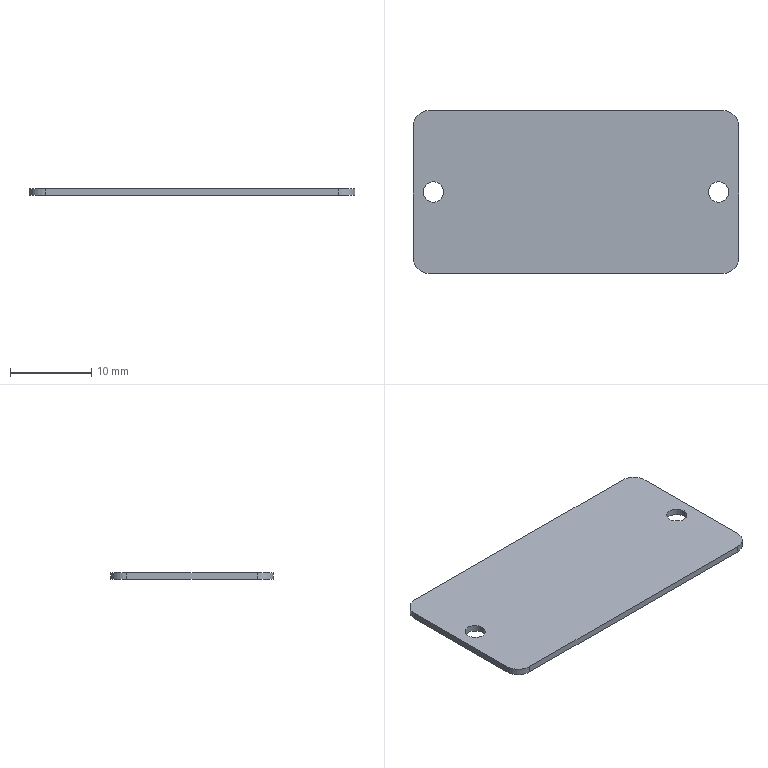Part | STEP file | [Nameplate]-1 | 1 solid | 14 faces | box 40 x 20 x 0.8 mm | volume 629.399 mm3 | cylinder 8 | plane 6 | commonest cylinder face diameters 2.5 x4 4 x4
STEP:
#1=CARTESIAN_POINT('',(38.75,10.,0.));
#2=VERTEX_POINT('',#1);
#3=CARTESIAN_POINT('',(36.25,10.,0.));
#4=VERTEX_POINT('',#3);
#5=CARTESIAN_POINT('',(37.5,10.,0.));
#6=DIRECTION('',(0.,0.,-1.));
#7=DIRECTION('',(-1.,0.,0.));
#8=AXIS2_PLACEMENT_3D('',#5,#6,#7);
#9=CIRCLE('',#8,1.25);
#10=EDGE_CURVE('',#2,#4,#9,.T.);
#11=ORIENTED_EDGE('',*,*,#10,.F.);
#12=CARTESIAN_POINT('',(38.75,10.,-0.8));
#13=VERTEX_POINT('',#12);
#14=CARTESIAN_POINT('',(38.75,10.,0.));
#15=DIRECTION('',(0.,0.,-1.));
#16=VECTOR('',#15,1000.);
#17=LINE('',#14,#16);
#18=EDGE_CURVE('',#2,#13,#17,.T.);
#19=ORIENTED_EDGE('',*,*,#18,.T.);
#20=CARTESIAN_POINT('',(36.25,10.,-0.8));
#21=VERTEX_POINT('',#20);
#22=CARTESIAN_POINT('',(37.5,10.,-0.8));
#23=DIRECTION('',(0.,0.,1.));
#24=DIRECTION('',(1.,0.,0.));
#25=AXIS2_PLACEMENT_3D('',#22,#23,#24);
#26=CIRCLE('',#25,1.25);
#27=EDGE_CURVE('',#21,#13,#26,.T.);
#28=ORIENTED_EDGE('',*,*,#27,.F.);
#29=CARTESIAN_POINT('',(36.25,10.,0.));
#30=DIRECTION('',(0.,0.,-1.));
#31=VECTOR('',#30,1000.);
#32=LINE('',#29,#31);
#33=EDGE_CURVE('',#4,#21,#32,.T.);
#34=ORIENTED_EDGE('',*,*,#33,.F.);
#35=EDGE_LOOP('',(#11,#19,#28,#34));
#36=FACE_OUTER_BOUND('',#35,.T.);
#37=CARTESIAN_POINT('',(37.5,10.,0.));
#38=DIRECTION('',(0.,0.,-1.));
#39=DIRECTION('',(-1.,0.,0.));
#40=AXIS2_PLACEMENT_3D('',#37,#38,#39);
#41=CYLINDRICAL_SURFACE('',#40,1.25);
#42=ADVANCED_FACE('',(#36),#41,.F.);
#43=CARTESIAN_POINT('',(3.75,10.,0.));
#44=VERTEX_POINT('',#43);
#45=CARTESIAN_POINT('',(1.25,10.,0.));
#46=VERTEX_POINT('',#45);
#47=CARTESIAN_POINT('',(2.5,10.,0.));
#48=DIRECTION('',(0.,0.,-1.));
#49=DIRECTION('',(-1.,0.,0.));
#50=AXIS2_PLACEMENT_3D('',#47,#48,#49);
#51=CIRCLE('',#50,1.25);
#52=EDGE_CURVE('',#44,#46,#51,.T.);
#53=ORIENTED_EDGE('',*,*,#52,.F.);
#54=CARTESIAN_POINT('',(3.75,10.,-0.8));
#55=VERTEX_POINT('',#54);
#56=CARTESIAN_POINT('',(3.75,10.,0.));
#57=DIRECTION('',(0.,0.,-1.));
#58=VECTOR('',#57,1000.);
#59=LINE('',#56,#58);
#60=EDGE_CURVE('',#44,#55,#59,.T.);
#61=ORIENTED_EDGE('',*,*,#60,.T.);
#62=CARTESIAN_POINT('',(1.25,10.,-0.8));
#63=VERTEX_POINT('',#62);
#64=CARTESIAN_POINT('',(2.5,10.,-0.8));
#65=DIRECTION('',(0.,0.,1.));
#66=DIRECTION('',(1.,0.,0.));
#67=AXIS2_PLACEMENT_3D('',#64,#65,#66);
#68=CIRCLE('',#67,1.25);
#69=EDGE_CURVE('',#63,#55,#68,.T.);
#70=ORIENTED_EDGE('',*,*,#69,.F.);
#71=CARTESIAN_POINT('',(1.25,10.,0.));
#72=DIRECTION('',(0.,0.,-1.));
#73=VECTOR('',#72,1000.);
#74=LINE('',#71,#73);
#75=EDGE_CURVE('',#46,#63,#74,.T.);
#76=ORIENTED_EDGE('',*,*,#75,.F.);
#77=EDGE_LOOP('',(#53,#61,#70,#76));
#78=FACE_OUTER_BOUND('',#77,.T.);
#79=CARTESIAN_POINT('',(2.5,10.,0.));
#80=DIRECTION('',(0.,0.,-1.));
#81=DIRECTION('',(-1.,0.,0.));
#82=AXIS2_PLACEMENT_3D('',#79,#80,#81);
#83=CYLINDRICAL_SURFACE('',#82,1.25);
#84=ADVANCED_FACE('',(#78),#83,.F.);
#85=CARTESIAN_POINT('',(38.,20.,0.));
#86=VERTEX_POINT('',#85);
#87=CARTESIAN_POINT('',(2.,20.,0.));
#88=VERTEX_POINT('',#87);
#89=CARTESIAN_POINT('',(38.,20.,0.));
#90=DIRECTION('',(-1.,0.,0.));
#91=VECTOR('',#90,1000.);
#92=LINE('',#89,#91);
#93=EDGE_CURVE('',#86,#88,#92,.T.);
#94=ORIENTED_EDGE('',*,*,#93,.F.);
#95=CARTESIAN_POINT('',(38.,20.,-0.8));
#96=VERTEX_POINT('',#95);
#97=CARTESIAN_POINT('',(38.,20.,-0.8));
#98=DIRECTION('',(0.,0.,1.));
#99=VECTOR('',#98,1000.);
#100=LINE('',#97,#99);
#101=EDGE_CURVE('',#96,#86,#100,.T.);
#102=ORIENTED_EDGE('',*,*,#101,.F.);
#103=CARTESIAN_POINT('',(2.,20.,-0.8));
#104=VERTEX_POINT('',#103);
#105=CARTESIAN_POINT('',(38.,20.,-0.8));
#106=DIRECTION('',(-1.,0.,0.));
#107=VECTOR('',#106,1000.);
#108=LINE('',#105,#107);
#109=EDGE_CURVE('',#96,#104,#108,.T.);
#110=ORIENTED_EDGE('',*,*,#109,.T.);
#111=CARTESIAN_POINT('',(2.,20.,-0.8));
#112=DIRECTION('',(0.,0.,1.));
#113=VECTOR('',#112,1000.);
#114=LINE('',#111,#113);
#115=EDGE_CURVE('',#104,#88,#114,.T.);
#116=ORIENTED_EDGE('',*,*,#115,.T.);
#117=EDGE_LOOP('',(#94,#102,#110,#116));
#118=FACE_OUTER_BOUND('',#117,.T.);
#119=CARTESIAN_POINT('',(38.,20.,-0.8));
#120=DIRECTION('',(0.,1.,0.));
#121=DIRECTION('',(-1.,0.,0.));
#122=AXIS2_PLACEMENT_3D('',#119,#120,#121);
#123=PLANE('',#122);
#124=ADVANCED_FACE('',(#118),#123,.T.);
#125=CARTESIAN_POINT('',(0.,18.,0.));
#126=VERTEX_POINT('',#125);
#127=CARTESIAN_POINT('',(2.,18.,0.));
#128=DIRECTION('',(0.,0.,1.));
#129=DIRECTION('',(1.,0.,0.));
#130=AXIS2_PLACEMENT_3D('',#127,#128,#129);
#131=CIRCLE('',#130,2.);
#132=EDGE_CURVE('',#88,#126,#131,.T.);
#133=ORIENTED_EDGE('',*,*,#132,.F.);
#134=ORIENTED_EDGE('',*,*,#115,.F.);
#135=CARTESIAN_POINT('',(0.,18.,-0.8));
#136=VERTEX_POINT('',#135);
#137=CARTESIAN_POINT('',(2.,18.,-0.8));
#138=DIRECTION('',(0.,0.,1.));
#139=DIRECTION('',(1.,0.,0.));
#140=AXIS2_PLACEMENT_3D('',#137,#138,#139);
#141=CIRCLE('',#140,2.);
#142=EDGE_CURVE('',#104,#136,#141,.T.);
#143=ORIENTED_EDGE('',*,*,#142,.T.);
#144=CARTESIAN_POINT('',(0.,18.,-0.8));
#145=DIRECTION('',(0.,0.,1.));
#146=VECTOR('',#145,1000.);
#147=LINE('',#144,#146);
#148=EDGE_CURVE('',#136,#126,#147,.T.);
#149=ORIENTED_EDGE('',*,*,#148,.T.);
#150=EDGE_LOOP('',(#133,#134,#143,#149));
#151=FACE_OUTER_BOUND('',#150,.T.);
#152=CARTESIAN_POINT('',(2.,18.,-0.8));
#153=DIRECTION('',(0.,0.,1.));
#154=DIRECTION('',(1.,0.,0.));
#155=AXIS2_PLACEMENT_3D('',#152,#153,#154);
#156=CYLINDRICAL_SURFACE('',#155,2.);
#157=ADVANCED_FACE('',(#151),#156,.T.);
#158=CARTESIAN_POINT('',(0.,2.,0.));
#159=VERTEX_POINT('',#158);
#160=CARTESIAN_POINT('',(0.,18.,0.));
#161=DIRECTION('',(0.,-1.,0.));
#162=VECTOR('',#161,1000.);
#163=LINE('',#160,#162);
#164=EDGE_CURVE('',#126,#159,#163,.T.);
#165=ORIENTED_EDGE('',*,*,#164,.F.);
#166=ORIENTED_EDGE('',*,*,#148,.F.);
#167=CARTESIAN_POINT('',(0.,2.,-0.8));
#168=VERTEX_POINT('',#167);
#169=CARTESIAN_POINT('',(0.,18.,-0.8));
#170=DIRECTION('',(0.,-1.,0.));
#171=VECTOR('',#170,1000.);
#172=LINE('',#169,#171);
#173=EDGE_CURVE('',#136,#168,#172,.T.);
#174=ORIENTED_EDGE('',*,*,#173,.T.);
#175=CARTESIAN_POINT('',(0.,2.,-0.8));
#176=DIRECTION('',(0.,0.,1.));
#177=VECTOR('',#176,1000.);
#178=LINE('',#175,#177);
#179=EDGE_CURVE('',#168,#159,#178,.T.);
#180=ORIENTED_EDGE('',*,*,#179,.T.);
#181=EDGE_LOOP('',(#165,#166,#174,#180));
#182=FACE_OUTER_BOUND('',#181,.T.);
#183=CARTESIAN_POINT('',(0.,18.,-0.8));
#184=DIRECTION('',(-1.,0.,0.));
#185=DIRECTION('',(0.,-1.,0.));
#186=AXIS2_PLACEMENT_3D('',#183,#184,#185);
#187=PLANE('',#186);
#188=ADVANCED_FACE('',(#182),#187,.T.);
#189=CARTESIAN_POINT('',(2.,0.,0.));
#190=VERTEX_POINT('',#189);
#191=CARTESIAN_POINT('',(2.,2.,0.));
#192=DIRECTION('',(0.,0.,1.));
#193=DIRECTION('',(1.,0.,0.));
#194=AXIS2_PLACEMENT_3D('',#191,#192,#193);
#195=CIRCLE('',#194,2.);
#196=EDGE_CURVE('',#159,#190,#195,.T.);
#197=ORIENTED_EDGE('',*,*,#196,.F.);
#198=ORIENTED_EDGE('',*,*,#179,.F.);
#199=CARTESIAN_POINT('',(2.,0.,-0.8));
#200=VERTEX_POINT('',#199);
#201=CARTESIAN_POINT('',(2.,2.,-0.8));
#202=DIRECTION('',(0.,0.,1.));
#203=DIRECTION('',(1.,0.,0.));
#204=AXIS2_PLACEMENT_3D('',#201,#202,#203);
#205=CIRCLE('',#204,2.);
#206=EDGE_CURVE('',#168,#200,#205,.T.);
#207=ORIENTED_EDGE('',*,*,#206,.T.);
#208=CARTESIAN_POINT('',(2.,0.,-0.8));
#209=DIRECTION('',(0.,0.,1.));
#210=VECTOR('',#209,1000.);
#211=LINE('',#208,#210);
#212=EDGE_CURVE('',#200,#190,#211,.T.);
#213=ORIENTED_EDGE('',*,*,#212,.T.);
#214=EDGE_LOOP('',(#197,#198,#207,#213));
#215=FACE_OUTER_BOUND('',#214,.T.);
#216=CARTESIAN_POINT('',(2.,2.,-0.8));
#217=DIRECTION('',(0.,0.,1.));
#218=DIRECTION('',(1.,0.,0.));
#219=AXIS2_PLACEMENT_3D('',#216,#217,#218);
#220=CYLINDRICAL_SURFACE('',#219,2.);
#221=ADVANCED_FACE('',(#215),#220,.T.);
#222=CARTESIAN_POINT('',(38.,0.,0.));
#223=VERTEX_POINT('',#222);
#224=CARTESIAN_POINT('',(2.,0.,0.));
#225=DIRECTION('',(1.,0.,0.));
#226=VECTOR('',#225,1000.);
#227=LINE('',#224,#226);
#228=EDGE_CURVE('',#190,#223,#227,.T.);
#229=ORIENTED_EDGE('',*,*,#228,.F.);
#230=ORIENTED_EDGE('',*,*,#212,.F.);
#231=CARTESIAN_POINT('',(38.,0.,-0.8));
#232=VERTEX_POINT('',#231);
#233=CARTESIAN_POINT('',(2.,0.,-0.8));
#234=DIRECTION('',(1.,0.,0.));
#235=VECTOR('',#234,1000.);
#236=LINE('',#233,#235);
#237=EDGE_CURVE('',#200,#232,#236,.T.);
#238=ORIENTED_EDGE('',*,*,#237,.T.);
#239=CARTESIAN_POINT('',(38.,0.,-0.8));
#240=DIRECTION('',(0.,0.,1.));
#241=VECTOR('',#240,1000.);
#242=LINE('',#239,#241);
#243=EDGE_CURVE('',#232,#223,#242,.T.);
#244=ORIENTED_EDGE('',*,*,#243,.T.);
#245=EDGE_LOOP('',(#229,#230,#238,#244));
#246=FACE_OUTER_BOUND('',#245,.T.);
#247=CARTESIAN_POINT('',(2.,0.,-0.8));
#248=DIRECTION('',(0.,-1.,0.));
#249=DIRECTION('',(0.,0.,-1.));
#250=AXIS2_PLACEMENT_3D('',#247,#248,#249);
#251=PLANE('',#250);
#252=ADVANCED_FACE('',(#246),#251,.T.);
#253=CARTESIAN_POINT('',(40.,2.,0.));
#254=VERTEX_POINT('',#253);
#255=CARTESIAN_POINT('',(38.,2.,0.));
#256=DIRECTION('',(0.,0.,1.));
#257=DIRECTION('',(1.,0.,0.));
#258=AXIS2_PLACEMENT_3D('',#255,#256,#257);
#259=CIRCLE('',#258,2.);
#260=EDGE_CURVE('',#223,#254,#259,.T.);
#261=ORIENTED_EDGE('',*,*,#260,.F.);
#262=ORIENTED_EDGE('',*,*,#243,.F.);
#263=CARTESIAN_POINT('',(40.,2.,-0.8));
#264=VERTEX_POINT('',#263);
#265=CARTESIAN_POINT('',(38.,2.,-0.8));
#266=DIRECTION('',(0.,0.,1.));
#267=DIRECTION('',(1.,0.,0.));
#268=AXIS2_PLACEMENT_3D('',#265,#266,#267);
#269=CIRCLE('',#268,2.);
#270=EDGE_CURVE('',#232,#264,#269,.T.);
#271=ORIENTED_EDGE('',*,*,#270,.T.);
#272=CARTESIAN_POINT('',(40.,2.,-0.8));
#273=DIRECTION('',(0.,0.,1.));
#274=VECTOR('',#273,1000.);
#275=LINE('',#272,#274);
#276=EDGE_CURVE('',#264,#254,#275,.T.);
#277=ORIENTED_EDGE('',*,*,#276,.T.);
#278=EDGE_LOOP('',(#261,#262,#271,#277));
#279=FACE_OUTER_BOUND('',#278,.T.);
#280=CARTESIAN_POINT('',(38.,2.,-0.8));
#281=DIRECTION('',(0.,0.,1.));
#282=DIRECTION('',(1.,0.,0.));
#283=AXIS2_PLACEMENT_3D('',#280,#281,#282);
#284=CYLINDRICAL_SURFACE('',#283,2.);
#285=ADVANCED_FACE('',(#279),#284,.T.);
#286=CARTESIAN_POINT('',(40.,18.,0.));
#287=VERTEX_POINT('',#286);
#288=CARTESIAN_POINT('',(40.,2.,0.));
#289=DIRECTION('',(0.,1.,0.));
#290=VECTOR('',#289,1000.);
#291=LINE('',#288,#290);
#292=EDGE_CURVE('',#254,#287,#291,.T.);
#293=ORIENTED_EDGE('',*,*,#292,.F.);
#294=ORIENTED_EDGE('',*,*,#276,.F.);
#295=CARTESIAN_POINT('',(40.,18.,-0.8));
#296=VERTEX_POINT('',#295);
#297=CARTESIAN_POINT('',(40.,2.,-0.8));
#298=DIRECTION('',(0.,1.,0.));
#299=VECTOR('',#298,1000.);
#300=LINE('',#297,#299);
#301=EDGE_CURVE('',#264,#296,#300,.T.);
#302=ORIENTED_EDGE('',*,*,#301,.T.);
#303=CARTESIAN_POINT('',(40.,18.,-0.8));
#304=DIRECTION('',(0.,0.,1.));
#305=VECTOR('',#304,1000.);
#306=LINE('',#303,#305);
#307=EDGE_CURVE('',#296,#287,#306,.T.);
#308=ORIENTED_EDGE('',*,*,#307,.T.);
#309=EDGE_LOOP('',(#293,#294,#302,#308));
#310=FACE_OUTER_BOUND('',#309,.T.);
#311=CARTESIAN_POINT('',(40.,2.,-0.8));
#312=DIRECTION('',(1.,0.,0.));
#313=DIRECTION('',(0.,0.,-1.));
#314=AXIS2_PLACEMENT_3D('',#311,#312,#313);
#315=PLANE('',#314);
#316=ADVANCED_FACE('',(#310),#315,.T.);
#317=CARTESIAN_POINT('',(38.,18.,0.));
#318=DIRECTION('',(0.,0.,1.));
#319=DIRECTION('',(1.,0.,0.));
#320=AXIS2_PLACEMENT_3D('',#317,#318,#319);
#321=CIRCLE('',#320,2.);
#322=EDGE_CURVE('',#287,#86,#321,.T.);
#323=ORIENTED_EDGE('',*,*,#322,.F.);
#324=ORIENTED_EDGE('',*,*,#307,.F.);
#325=CARTESIAN_POINT('',(38.,18.,-0.8));
#326=DIRECTION('',(0.,0.,1.));
#327=DIRECTION('',(1.,0.,0.));
#328=AXIS2_PLACEMENT_3D('',#325,#326,#327);
#329=CIRCLE('',#328,2.);
#330=EDGE_CURVE('',#296,#96,#329,.T.);
#331=ORIENTED_EDGE('',*,*,#330,.T.);
#332=ORIENTED_EDGE('',*,*,#101,.T.);
#333=EDGE_LOOP('',(#323,#324,#331,#332));
#334=FACE_OUTER_BOUND('',#333,.T.);
#335=CARTESIAN_POINT('',(38.,18.,-0.8));
#336=DIRECTION('',(0.,0.,1.));
#337=DIRECTION('',(1.,0.,0.));
#338=AXIS2_PLACEMENT_3D('',#335,#336,#337);
#339=CYLINDRICAL_SURFACE('',#338,2.);
#340=ADVANCED_FACE('',(#334),#339,.T.);
#341=ORIENTED_EDGE('',*,*,#27,.T.);
#342=CARTESIAN_POINT('',(37.5,10.,-0.8));
#343=DIRECTION('',(0.,0.,1.));
#344=DIRECTION('',(1.,0.,0.));
#345=AXIS2_PLACEMENT_3D('',#342,#343,#344);
#346=CIRCLE('',#345,1.25);
#347=EDGE_CURVE('',#13,#21,#346,.T.);
#348=ORIENTED_EDGE('',*,*,#347,.T.);
#349=EDGE_LOOP('',(#341,#348));
#350=FACE_BOUND('',#349,.T.);
#351=ORIENTED_EDGE('',*,*,#69,.T.);
#352=CARTESIAN_POINT('',(2.5,10.,-0.8));
#353=DIRECTION('',(0.,0.,1.));
#354=DIRECTION('',(1.,0.,0.));
#355=AXIS2_PLACEMENT_3D('',#352,#353,#354);
#356=CIRCLE('',#355,1.25);
#357=EDGE_CURVE('',#55,#63,#356,.T.);
#358=ORIENTED_EDGE('',*,*,#357,.T.);
#359=EDGE_LOOP('',(#351,#358));
#360=FACE_BOUND('',#359,.T.);
#361=ORIENTED_EDGE('',*,*,#109,.F.);
#362=ORIENTED_EDGE('',*,*,#330,.F.);
#363=ORIENTED_EDGE('',*,*,#301,.F.);
#364=ORIENTED_EDGE('',*,*,#270,.F.);
#365=ORIENTED_EDGE('',*,*,#237,.F.);
#366=ORIENTED_EDGE('',*,*,#206,.F.);
#367=ORIENTED_EDGE('',*,*,#173,.F.);
#368=ORIENTED_EDGE('',*,*,#142,.F.);
#369=EDGE_LOOP('',(#361,#362,#363,#364,#365,#366,#367,#368));
#370=FACE_OUTER_BOUND('',#369,.T.);
#371=CARTESIAN_POINT('',(2.,18.,-0.8));
#372=DIRECTION('',(0.,0.,1.));
#373=DIRECTION('',(1.,0.,0.));
#374=AXIS2_PLACEMENT_3D('',#371,#372,#373);
#375=PLANE('',#374);
#376=ADVANCED_FACE('',(#350,#360,#370),#375,.F.);
#377=CARTESIAN_POINT('',(37.5,10.,0.));
#378=DIRECTION('',(0.,0.,-1.));
#379=DIRECTION('',(-1.,0.,0.));
#380=AXIS2_PLACEMENT_3D('',#377,#378,#379);
#381=CIRCLE('',#380,1.25);
#382=EDGE_CURVE('',#4,#2,#381,.T.);
#383=ORIENTED_EDGE('',*,*,#382,.T.);
#384=ORIENTED_EDGE('',*,*,#10,.T.);
#385=EDGE_LOOP('',(#383,#384));
#386=FACE_BOUND('',#385,.T.);
#387=CARTESIAN_POINT('',(2.5,10.,0.));
#388=DIRECTION('',(0.,0.,-1.));
#389=DIRECTION('',(-1.,0.,0.));
#390=AXIS2_PLACEMENT_3D('',#387,#388,#389);
#391=CIRCLE('',#390,1.25);
#392=EDGE_CURVE('',#46,#44,#391,.T.);
#393=ORIENTED_EDGE('',*,*,#392,.T.);
#394=ORIENTED_EDGE('',*,*,#52,.T.);
#395=EDGE_LOOP('',(#393,#394));
#396=FACE_BOUND('',#395,.T.);
#397=ORIENTED_EDGE('',*,*,#93,.T.);
#398=ORIENTED_EDGE('',*,*,#132,.T.);
#399=ORIENTED_EDGE('',*,*,#164,.T.);
#400=ORIENTED_EDGE('',*,*,#196,.T.);
#401=ORIENTED_EDGE('',*,*,#228,.T.);
#402=ORIENTED_EDGE('',*,*,#260,.T.);
#403=ORIENTED_EDGE('',*,*,#292,.T.);
#404=ORIENTED_EDGE('',*,*,#322,.T.);
#405=EDGE_LOOP('',(#397,#398,#399,#400,#401,#402,#403,#404));
#406=FACE_OUTER_BOUND('',#405,.T.);
#407=CARTESIAN_POINT('',(2.,18.,0.));
#408=DIRECTION('',(0.,0.,1.));
#409=DIRECTION('',(1.,0.,0.));
#410=AXIS2_PLACEMENT_3D('',#407,#408,#409);
#411=PLANE('',#410);
#412=ADVANCED_FACE('',(#386,#396,#406),#411,.T.);
#413=ORIENTED_EDGE('',*,*,#60,.F.);
#414=ORIENTED_EDGE('',*,*,#392,.F.);
#415=ORIENTED_EDGE('',*,*,#75,.T.);
#416=ORIENTED_EDGE('',*,*,#357,.F.);
#417=EDGE_LOOP('',(#413,#414,#415,#416));
#418=FACE_OUTER_BOUND('',#417,.T.);
#419=CARTESIAN_POINT('',(2.5,10.,0.));
#420=DIRECTION('',(0.,0.,-1.));
#421=DIRECTION('',(-1.,0.,0.));
#422=AXIS2_PLACEMENT_3D('',#419,#420,#421);
#423=CYLINDRICAL_SURFACE('',#422,1.25);
#424=ADVANCED_FACE('',(#418),#423,.F.);
#425=ORIENTED_EDGE('',*,*,#18,.F.);
#426=ORIENTED_EDGE('',*,*,#382,.F.);
#427=ORIENTED_EDGE('',*,*,#33,.T.);
#428=ORIENTED_EDGE('',*,*,#347,.F.);
#429=EDGE_LOOP('',(#425,#426,#427,#428));
#430=FACE_OUTER_BOUND('',#429,.T.);
#431=CARTESIAN_POINT('',(37.5,10.,0.));
#432=DIRECTION('',(0.,0.,-1.));
#433=DIRECTION('',(-1.,0.,0.));
#434=AXIS2_PLACEMENT_3D('',#431,#432,#433);
#435=CYLINDRICAL_SURFACE('',#434,1.25);
#436=ADVANCED_FACE('',(#430),#435,.F.);
#437=CLOSED_SHELL('',(#42,#84,#124,#157,#188,#221,#252,#285,#316,#340,#376,#412,#424,#436));
#438=MANIFOLD_SOLID_BREP('',#437);
#439=CARTESIAN_POINT('',(0.,0.,0.));
#440=DIRECTION('',(0.,0.,1.));
#441=DIRECTION('',(1.,0.,0.));
#442=AXIS2_PLACEMENT_3D('',#439,#440,#441);
#443=(LENGTH_UNIT()NAMED_UNIT(*)SI_UNIT(.MILLI.,.METRE.));
#444=UNCERTAINTY_MEASURE_WITH_UNIT(LENGTH_MEASURE(0.00001),#443,'','');
#445=(NAMED_UNIT(*)PLANE_ANGLE_UNIT()SI_UNIT($,.RADIAN.));
#446=(NAMED_UNIT(*)SI_UNIT($,.STERADIAN.)SOLID_ANGLE_UNIT());
#447=(GEOMETRIC_REPRESENTATION_CONTEXT(3)GLOBAL_UNCERTAINTY_ASSIGNED_CONTEXT((#444))GLOBAL_UNIT_ASSIGNED_CONTEXT((#443,#445,#446))REPRESENTATION_CONTEXT('',''));
#448=ADVANCED_BREP_SHAPE_REPRESENTATION('',(#438,#442),#447);